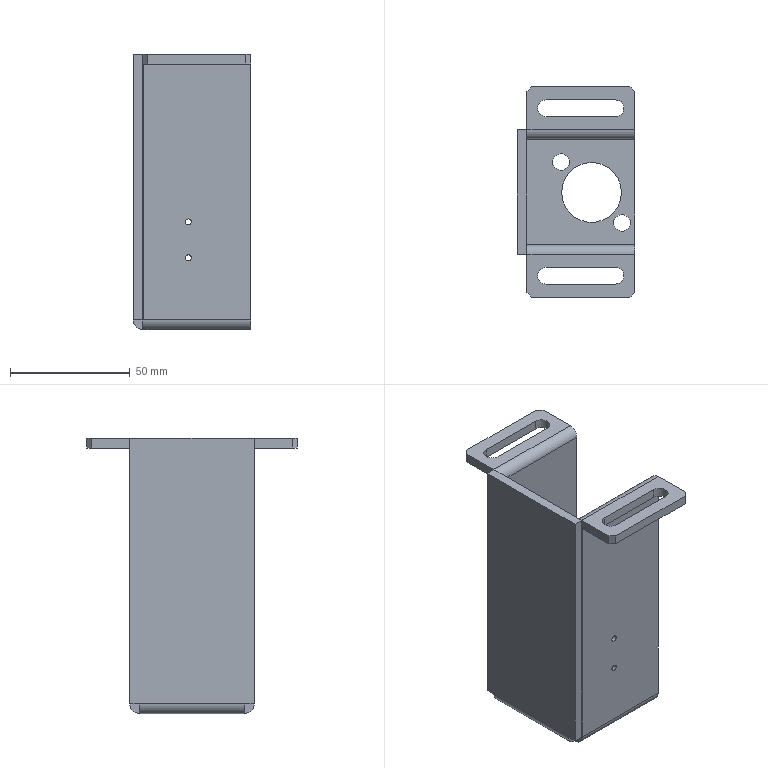Part | STEP file | 1 solid | 88 faces | box 49.01 x 88 x 115 mm | volume 72509 mm3 | plane 54 | cylinder 34 | commonest cylinder face diameters 7 x10 2.5 x8 0.02 x5 8.02 x5 4 x4 25 x2